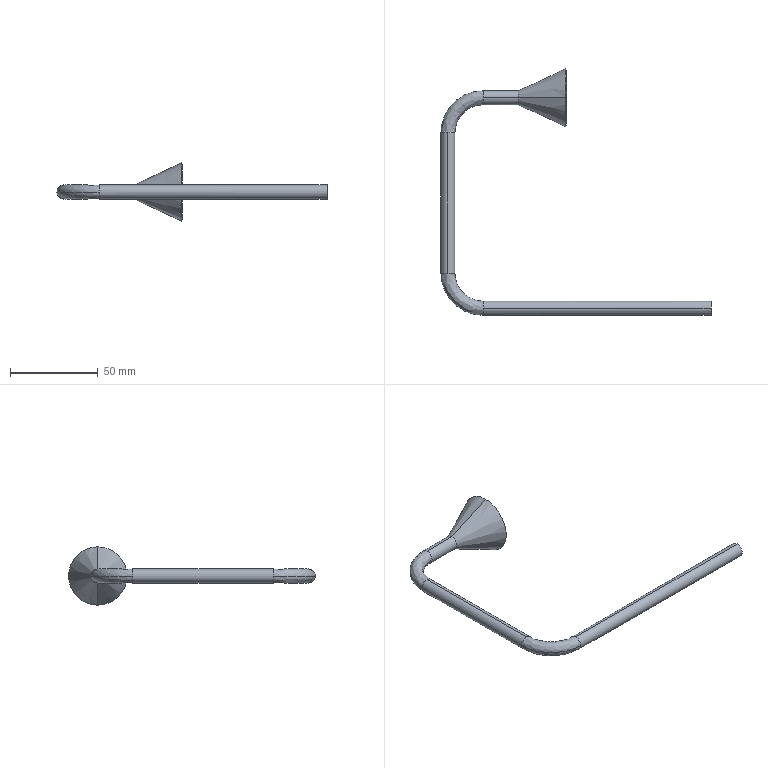Part | STEP file | 750038201 | 1 solid | 27 faces | box 154 x 140.678 x 33.357 mm | volume 8140 mm3 | cylinder 12 | spline 8 | cone 6 | plane 1 | commonest cylinder face diameters 6 x6 8 x6
STEP:
#1=CARTESIAN_POINT('',(20.,4.,0.));
#2=VERTEX_POINT('',#1);
#3=CARTESIAN_POINT('',(20.,0.,4.));
#4=VERTEX_POINT('',#3);
#5=CARTESIAN_POINT('',(20.,0.,0.));
#6=DIRECTION('',(1.,0.,0.));
#7=DIRECTION('',(0.,0.,-1.));
#8=AXIS2_PLACEMENT_3D('',#5,#6,#7);
#9=CIRCLE('',#8,4.);
#10=EDGE_CURVE('',#2,#4,#9,.T.);
#11=ORIENTED_EDGE('',*,*,#10,.T.);
#12=CARTESIAN_POINT('',(150.,0.,4.));
#13=VERTEX_POINT('',#12);
#14=CARTESIAN_POINT('',(20.,0.,4.));
#15=DIRECTION('',(1.,0.,0.));
#16=VECTOR('',#15,1000.);
#17=LINE('',#14,#16);
#18=EDGE_CURVE('',#4,#13,#17,.T.);
#19=ORIENTED_EDGE('',*,*,#18,.T.);
#20=CARTESIAN_POINT('',(150.,0.,-4.));
#21=VERTEX_POINT('',#20);
#22=CARTESIAN_POINT('',(150.,0.,0.));
#23=DIRECTION('',(-1.,0.,0.));
#24=DIRECTION('',(0.,0.,-1.));
#25=AXIS2_PLACEMENT_3D('',#22,#23,#24);
#26=CIRCLE('',#25,4.);
#27=EDGE_CURVE('',#13,#21,#26,.T.);
#28=ORIENTED_EDGE('',*,*,#27,.T.);
#29=CARTESIAN_POINT('',(20.,0.,-4.));
#30=VERTEX_POINT('',#29);
#31=CARTESIAN_POINT('',(20.,0.,-4.));
#32=DIRECTION('',(1.,0.,0.));
#33=VECTOR('',#32,1000.);
#34=LINE('',#31,#33);
#35=EDGE_CURVE('',#30,#21,#34,.T.);
#36=ORIENTED_EDGE('',*,*,#35,.F.);
#37=CARTESIAN_POINT('',(20.,0.,0.));
#38=DIRECTION('',(1.,0.,0.));
#39=DIRECTION('',(0.,0.,-1.));
#40=AXIS2_PLACEMENT_3D('',#37,#38,#39);
#41=CIRCLE('',#40,4.);
#42=EDGE_CURVE('',#30,#2,#41,.T.);
#43=ORIENTED_EDGE('',*,*,#42,.T.);
#44=EDGE_LOOP('',(#11,#19,#28,#36,#43));
#45=FACE_OUTER_BOUND('',#44,.T.);
#46=CARTESIAN_POINT('',(20.,0.,0.));
#47=DIRECTION('',(1.,0.,0.));
#48=DIRECTION('',(0.,0.,-1.));
#49=AXIS2_PLACEMENT_3D('',#46,#47,#48);
#50=CYLINDRICAL_SURFACE('',#49,4.);
#51=ADVANCED_FACE('',(#45),#50,.T.);
#52=ORIENTED_EDGE('',*,*,#10,.F.);
#53=CARTESIAN_POINT('',(4.,20.,0.));
#54=VERTEX_POINT('',#53);
#55=CARTESIAN_POINT('',(20.,20.,0.));
#56=DIRECTION('',(0.,0.,-1.));
#57=DIRECTION('',(-1.,0.,0.));
#58=AXIS2_PLACEMENT_3D('',#55,#56,#57);
#59=CIRCLE('',#58,16.);
#60=EDGE_CURVE('',#2,#54,#59,.T.);
#61=ORIENTED_EDGE('',*,*,#60,.T.);
#62=CARTESIAN_POINT('',(0.,20.,4.));
#63=VERTEX_POINT('',#62);
#64=CARTESIAN_POINT('',(0.,20.,0.));
#65=DIRECTION('',(0.,-1.,0.));
#66=DIRECTION('',(-1.,0.,0.));
#67=AXIS2_PLACEMENT_3D('',#64,#65,#66);
#68=CIRCLE('',#67,4.);
#69=EDGE_CURVE('',#54,#63,#68,.T.);
#70=ORIENTED_EDGE('',*,*,#69,.T.);
#71=CARTESIAN_POINT('',(-4.,20.,0.));
#72=VERTEX_POINT('',#71);
#73=CARTESIAN_POINT('',(0.,20.,0.));
#74=DIRECTION('',(0.,-1.,0.));
#75=DIRECTION('',(-1.,0.,0.));
#76=AXIS2_PLACEMENT_3D('',#73,#74,#75);
#77=CIRCLE('',#76,4.);
#78=EDGE_CURVE('',#63,#72,#77,.T.);
#79=ORIENTED_EDGE('',*,*,#78,.T.);
#80=CARTESIAN_POINT('',(20.,-4.,0.));
#81=VERTEX_POINT('',#80);
#82=CARTESIAN_POINT('',(20.,20.,0.));
#83=DIRECTION('',(0.,0.,-1.));
#84=DIRECTION('',(-1.,0.,0.));
#85=AXIS2_PLACEMENT_3D('',#82,#83,#84);
#86=CIRCLE('',#85,24.);
#87=EDGE_CURVE('',#81,#72,#86,.T.);
#88=ORIENTED_EDGE('',*,*,#87,.F.);
#89=CARTESIAN_POINT('',(20.,0.,0.));
#90=DIRECTION('',(1.,0.,0.));
#91=DIRECTION('',(0.,0.,-1.));
#92=AXIS2_PLACEMENT_3D('',#89,#90,#91);
#93=CIRCLE('',#92,4.);
#94=EDGE_CURVE('',#4,#81,#93,.T.);
#95=ORIENTED_EDGE('',*,*,#94,.F.);
#96=EDGE_LOOP('',(#52,#61,#70,#79,#88,#95));
#97=FACE_OUTER_BOUND('',#96,.T.);
#98=CARTESIAN_POINT('',(20.,-4.,0.));
#99=CARTESIAN_POINT('',(5.941,-4.,0.));
#100=CARTESIAN_POINT('',(-4.,5.941,0.));
#101=CARTESIAN_POINT('',(-4.,20.,0.));
#102=CARTESIAN_POINT('',(20.,-4.,8.));
#103=CARTESIAN_POINT('',(5.941,-4.,8.));
#104=CARTESIAN_POINT('',(-4.,5.941,8.));
#105=CARTESIAN_POINT('',(-4.,20.,8.));
#106=CARTESIAN_POINT('',(20.,4.,8.));
#107=CARTESIAN_POINT('',(10.627,4.,8.));
#108=CARTESIAN_POINT('',(4.,10.627,8.));
#109=CARTESIAN_POINT('',(4.,20.,8.));
#110=CARTESIAN_POINT('',(20.,4.,0.));
#111=CARTESIAN_POINT('',(10.627,4.,0.));
#112=CARTESIAN_POINT('',(4.,10.627,0.));
#113=CARTESIAN_POINT('',(4.,20.,0.));
#114=(BOUNDED_SURFACE()B_SPLINE_SURFACE(3,3,((#98,#99,#100,#101),(#102,#103,#104,#105),(#106,#107,#108,#109),(#110,#111,#112,#113)),.UNSPECIFIED.,.F.,.F.,.F.)B_SPLINE_SURFACE_WITH_KNOTS((4,4),(4,4),(0.,1.),(0.,1.),.UNSPECIFIED.)GEOMETRIC_REPRESENTATION_ITEM()RATIONAL_B_SPLINE_SURFACE(((1.,0.8047,0.8047,1.),(0.3333,0.2682,0.2682,0.3333),(0.3333,0.2682,0.2682,0.3333),(1.,0.8047,0.8047,1.)))REPRESENTATION_ITEM('')SURFACE());
#115=ADVANCED_FACE('',(#97),#114,.T.);
#116=CARTESIAN_POINT('',(20.,0.,3.));
#117=VERTEX_POINT('',#116);
#118=CARTESIAN_POINT('',(20.,-3.,0.));
#119=VERTEX_POINT('',#118);
#120=CARTESIAN_POINT('',(20.,0.,0.));
#121=DIRECTION('',(1.,0.,0.));
#122=DIRECTION('',(0.,0.,-1.));
#123=AXIS2_PLACEMENT_3D('',#120,#121,#122);
#124=CIRCLE('',#123,3.);
#125=EDGE_CURVE('',#117,#119,#124,.T.);
#126=ORIENTED_EDGE('',*,*,#125,.F.);
#127=CARTESIAN_POINT('',(150.,0.,3.));
#128=VERTEX_POINT('',#127);
#129=CARTESIAN_POINT('',(20.,0.,3.));
#130=DIRECTION('',(1.,0.,0.));
#131=VECTOR('',#130,1000.);
#132=LINE('',#129,#131);
#133=EDGE_CURVE('',#117,#128,#132,.T.);
#134=ORIENTED_EDGE('',*,*,#133,.T.);
#135=CARTESIAN_POINT('',(150.,0.,-3.));
#136=VERTEX_POINT('',#135);
#137=CARTESIAN_POINT('',(150.,0.,0.));
#138=DIRECTION('',(1.,0.,0.));
#139=DIRECTION('',(0.,0.,-1.));
#140=AXIS2_PLACEMENT_3D('',#137,#138,#139);
#141=CIRCLE('',#140,3.);
#142=EDGE_CURVE('',#128,#136,#141,.T.);
#143=ORIENTED_EDGE('',*,*,#142,.T.);
#144=CARTESIAN_POINT('',(20.,0.,-3.));
#145=VERTEX_POINT('',#144);
#146=CARTESIAN_POINT('',(20.,0.,-3.));
#147=DIRECTION('',(1.,0.,0.));
#148=VECTOR('',#147,1000.);
#149=LINE('',#146,#148);
#150=EDGE_CURVE('',#145,#136,#149,.T.);
#151=ORIENTED_EDGE('',*,*,#150,.F.);
#152=CARTESIAN_POINT('',(20.,0.,0.));
#153=DIRECTION('',(1.,0.,0.));
#154=DIRECTION('',(0.,0.,-1.));
#155=AXIS2_PLACEMENT_3D('',#152,#153,#154);
#156=CIRCLE('',#155,3.);
#157=EDGE_CURVE('',#119,#145,#156,.T.);
#158=ORIENTED_EDGE('',*,*,#157,.F.);
#159=EDGE_LOOP('',(#126,#134,#143,#151,#158));
#160=FACE_OUTER_BOUND('',#159,.T.);
#161=CARTESIAN_POINT('',(20.,0.,0.));
#162=DIRECTION('',(1.,0.,0.));
#163=DIRECTION('',(0.,0.,-1.));
#164=AXIS2_PLACEMENT_3D('',#161,#162,#163);
#165=CYLINDRICAL_SURFACE('',#164,3.);
#166=ADVANCED_FACE('',(#160),#165,.F.);
#167=CARTESIAN_POINT('',(0.,20.,-4.));
#168=VERTEX_POINT('',#167);
#169=CARTESIAN_POINT('',(0.,20.,0.));
#170=DIRECTION('',(0.,-1.,0.));
#171=DIRECTION('',(-1.,0.,0.));
#172=AXIS2_PLACEMENT_3D('',#169,#170,#171);
#173=CIRCLE('',#172,4.);
#174=EDGE_CURVE('',#168,#54,#173,.T.);
#175=ORIENTED_EDGE('',*,*,#174,.F.);
#176=CARTESIAN_POINT('',(0.,100.,-4.));
#177=VERTEX_POINT('',#176);
#178=CARTESIAN_POINT('',(0.,20.,-4.));
#179=DIRECTION('',(0.,1.,0.));
#180=VECTOR('',#179,1000.);
#181=LINE('',#178,#180);
#182=EDGE_CURVE('',#168,#177,#181,.T.);
#183=ORIENTED_EDGE('',*,*,#182,.T.);
#184=CARTESIAN_POINT('',(4.,100.,0.));
#185=VERTEX_POINT('',#184);
#186=CARTESIAN_POINT('',(0.,100.,0.));
#187=DIRECTION('',(0.,-1.,0.));
#188=DIRECTION('',(0.,0.,1.));
#189=AXIS2_PLACEMENT_3D('',#186,#187,#188);
#190=CIRCLE('',#189,4.);
#191=EDGE_CURVE('',#177,#185,#190,.T.);
#192=ORIENTED_EDGE('',*,*,#191,.T.);
#193=CARTESIAN_POINT('',(0.,100.,4.));
#194=VERTEX_POINT('',#193);
#195=CARTESIAN_POINT('',(0.,100.,0.));
#196=DIRECTION('',(0.,-1.,0.));
#197=DIRECTION('',(0.,0.,1.));
#198=AXIS2_PLACEMENT_3D('',#195,#196,#197);
#199=CIRCLE('',#198,4.);
#200=EDGE_CURVE('',#185,#194,#199,.T.);
#201=ORIENTED_EDGE('',*,*,#200,.T.);
#202=CARTESIAN_POINT('',(0.,20.,4.));
#203=DIRECTION('',(0.,1.,0.));
#204=VECTOR('',#203,1000.);
#205=LINE('',#202,#204);
#206=EDGE_CURVE('',#63,#194,#205,.T.);
#207=ORIENTED_EDGE('',*,*,#206,.F.);
#208=ORIENTED_EDGE('',*,*,#69,.F.);
#209=EDGE_LOOP('',(#175,#183,#192,#201,#207,#208));
#210=FACE_OUTER_BOUND('',#209,.T.);
#211=CARTESIAN_POINT('',(0.,20.,0.));
#212=DIRECTION('',(0.,1.,0.));
#213=DIRECTION('',(0.,0.,1.));
#214=AXIS2_PLACEMENT_3D('',#211,#212,#213);
#215=CYLINDRICAL_SURFACE('',#214,4.);
#216=ADVANCED_FACE('',(#210),#215,.T.);
#217=ORIENTED_EDGE('',*,*,#157,.T.);
#218=CARTESIAN_POINT('',(20.,3.,0.));
#219=VERTEX_POINT('',#218);
#220=CARTESIAN_POINT('',(20.,0.,0.));
#221=DIRECTION('',(1.,0.,0.));
#222=DIRECTION('',(0.,0.,-1.));
#223=AXIS2_PLACEMENT_3D('',#220,#221,#222);
#224=CIRCLE('',#223,3.);
#225=EDGE_CURVE('',#145,#219,#224,.T.);
#226=ORIENTED_EDGE('',*,*,#225,.T.);
#227=CARTESIAN_POINT('',(3.,20.,0.));
#228=VERTEX_POINT('',#227);
#229=CARTESIAN_POINT('',(20.,20.,0.));
#230=DIRECTION('',(0.,0.,-1.));
#231=DIRECTION('',(-1.,0.,0.));
#232=AXIS2_PLACEMENT_3D('',#229,#230,#231);
#233=CIRCLE('',#232,17.);
#234=EDGE_CURVE('',#219,#228,#233,.T.);
#235=ORIENTED_EDGE('',*,*,#234,.T.);
#236=CARTESIAN_POINT('',(0.,20.,-3.));
#237=VERTEX_POINT('',#236);
#238=CARTESIAN_POINT('',(0.,20.,0.));
#239=DIRECTION('',(0.,-1.,0.));
#240=DIRECTION('',(-1.,0.,0.));
#241=AXIS2_PLACEMENT_3D('',#238,#239,#240);
#242=CIRCLE('',#241,3.);
#243=EDGE_CURVE('',#237,#228,#242,.T.);
#244=ORIENTED_EDGE('',*,*,#243,.F.);
#245=CARTESIAN_POINT('',(-3.,20.,0.));
#246=VERTEX_POINT('',#245);
#247=CARTESIAN_POINT('',(0.,20.,0.));
#248=DIRECTION('',(0.,-1.,0.));
#249=DIRECTION('',(-1.,0.,0.));
#250=AXIS2_PLACEMENT_3D('',#247,#248,#249);
#251=CIRCLE('',#250,3.);
#252=EDGE_CURVE('',#246,#237,#251,.T.);
#253=ORIENTED_EDGE('',*,*,#252,.F.);
#254=CARTESIAN_POINT('',(20.,20.,0.));
#255=DIRECTION('',(0.,0.,-1.));
#256=DIRECTION('',(-1.,0.,0.));
#257=AXIS2_PLACEMENT_3D('',#254,#255,#256);
#258=CIRCLE('',#257,23.);
#259=EDGE_CURVE('',#119,#246,#258,.T.);
#260=ORIENTED_EDGE('',*,*,#259,.F.);
#261=EDGE_LOOP('',(#217,#226,#235,#244,#253,#260));
#262=FACE_OUTER_BOUND('',#261,.T.);
#263=CARTESIAN_POINT('',(20.,3.,0.));
#264=CARTESIAN_POINT('',(10.042,3.,0.));
#265=CARTESIAN_POINT('',(3.,10.042,0.));
#266=CARTESIAN_POINT('',(3.,20.,0.));
#267=CARTESIAN_POINT('',(20.,3.,-6.));
#268=CARTESIAN_POINT('',(10.042,3.,-6.));
#269=CARTESIAN_POINT('',(3.,10.042,-6.));
#270=CARTESIAN_POINT('',(3.,20.,-6.));
#271=CARTESIAN_POINT('',(20.,-3.,-6.));
#272=CARTESIAN_POINT('',(6.527,-3.,-6.));
#273=CARTESIAN_POINT('',(-3.,6.527,-6.));
#274=CARTESIAN_POINT('',(-3.,20.,-6.));
#275=CARTESIAN_POINT('',(20.,-3.,0.));
#276=CARTESIAN_POINT('',(6.527,-3.,0.));
#277=CARTESIAN_POINT('',(-3.,6.527,0.));
#278=CARTESIAN_POINT('',(-3.,20.,0.));
#279=(BOUNDED_SURFACE()B_SPLINE_SURFACE(3,3,((#263,#264,#265,#266),(#267,#268,#269,#270),(#271,#272,#273,#274),(#275,#276,#277,#278)),.UNSPECIFIED.,.F.,.F.,.F.)B_SPLINE_SURFACE_WITH_KNOTS((4,4),(4,4),(0.,1.),(0.,1.),.UNSPECIFIED.)GEOMETRIC_REPRESENTATION_ITEM()RATIONAL_B_SPLINE_SURFACE(((1.,0.8047,0.8047,1.),(0.3333,0.2682,0.2682,0.3333),(0.3333,0.2682,0.2682,0.3333),(1.,0.8047,0.8047,1.)))REPRESENTATION_ITEM('')SURFACE());
#280=ADVANCED_FACE('',(#262),#279,.F.);
#281=ORIENTED_EDGE('',*,*,#200,.F.);
#282=CARTESIAN_POINT('',(20.,116.,0.));
#283=VERTEX_POINT('',#282);
#284=CARTESIAN_POINT('',(20.,100.,0.));
#285=DIRECTION('',(0.,0.,-1.));
#286=DIRECTION('',(-1.,0.,0.));
#287=AXIS2_PLACEMENT_3D('',#284,#285,#286);
#288=CIRCLE('',#287,16.);
#289=EDGE_CURVE('',#185,#283,#288,.T.);
#290=ORIENTED_EDGE('',*,*,#289,.T.);
#291=CARTESIAN_POINT('',(20.,120.,4.));
#292=VERTEX_POINT('',#291);
#293=CARTESIAN_POINT('',(20.,120.,0.));
#294=DIRECTION('',(-1.,0.,0.));
#295=DIRECTION('',(0.,1.,0.));
#296=AXIS2_PLACEMENT_3D('',#293,#294,#295);
#297=CIRCLE('',#296,4.);
#298=EDGE_CURVE('',#283,#292,#297,.T.);
#299=ORIENTED_EDGE('',*,*,#298,.T.);
#300=CARTESIAN_POINT('',(20.,124.,0.));
#301=VERTEX_POINT('',#300);
#302=CARTESIAN_POINT('',(20.,120.,0.));
#303=DIRECTION('',(-1.,0.,0.));
#304=DIRECTION('',(0.,1.,0.));
#305=AXIS2_PLACEMENT_3D('',#302,#303,#304);
#306=CIRCLE('',#305,4.);
#307=EDGE_CURVE('',#292,#301,#306,.T.);
#308=ORIENTED_EDGE('',*,*,#307,.T.);
#309=CARTESIAN_POINT('',(-4.,100.,0.));
#310=VERTEX_POINT('',#309);
#311=CARTESIAN_POINT('',(20.,100.,0.));
#312=DIRECTION('',(0.,0.,-1.));
#313=DIRECTION('',(-1.,0.,0.));
#314=AXIS2_PLACEMENT_3D('',#311,#312,#313);
#315=CIRCLE('',#314,24.);
#316=EDGE_CURVE('',#310,#301,#315,.T.);
#317=ORIENTED_EDGE('',*,*,#316,.F.);
#318=CARTESIAN_POINT('',(0.,100.,0.));
#319=DIRECTION('',(0.,-1.,0.));
#320=DIRECTION('',(0.,0.,1.));
#321=AXIS2_PLACEMENT_3D('',#318,#319,#320);
#322=CIRCLE('',#321,4.);
#323=EDGE_CURVE('',#194,#310,#322,.T.);
#324=ORIENTED_EDGE('',*,*,#323,.F.);
#325=EDGE_LOOP('',(#281,#290,#299,#308,#317,#324));
#326=FACE_OUTER_BOUND('',#325,.T.);
#327=CARTESIAN_POINT('',(-4.,100.,0.));
#328=CARTESIAN_POINT('',(-4.,114.059,0.));
#329=CARTESIAN_POINT('',(5.941,124.,0.));
#330=CARTESIAN_POINT('',(20.,124.,0.));
#331=CARTESIAN_POINT('',(-4.,100.,8.));
#332=CARTESIAN_POINT('',(-4.,114.059,8.));
#333=CARTESIAN_POINT('',(5.941,124.,8.));
#334=CARTESIAN_POINT('',(20.,124.,8.));
#335=CARTESIAN_POINT('',(4.,100.,8.));
#336=CARTESIAN_POINT('',(4.,109.373,8.));
#337=CARTESIAN_POINT('',(10.627,116.,8.));
#338=CARTESIAN_POINT('',(20.,116.,8.));
#339=CARTESIAN_POINT('',(4.,100.,0.));
#340=CARTESIAN_POINT('',(4.,109.373,0.));
#341=CARTESIAN_POINT('',(10.627,116.,0.));
#342=CARTESIAN_POINT('',(20.,116.,0.));
#343=(BOUNDED_SURFACE()B_SPLINE_SURFACE(3,3,((#327,#328,#329,#330),(#331,#332,#333,#334),(#335,#336,#337,#338),(#339,#340,#341,#342)),.UNSPECIFIED.,.F.,.F.,.F.)B_SPLINE_SURFACE_WITH_KNOTS((4,4),(4,4),(0.,1.),(0.,1.),.UNSPECIFIED.)GEOMETRIC_REPRESENTATION_ITEM()RATIONAL_B_SPLINE_SURFACE(((1.,0.8047,0.8047,1.),(0.3333,0.2682,0.2682,0.3333),(0.3333,0.2682,0.2682,0.3333),(1.,0.8047,0.8047,1.)))REPRESENTATION_ITEM('')SURFACE());
#344=ADVANCED_FACE('',(#326),#343,.T.);
#345=CARTESIAN_POINT('',(0.,20.,3.));
#346=VERTEX_POINT('',#345);
#347=CARTESIAN_POINT('',(0.,20.,0.));
#348=DIRECTION('',(0.,-1.,0.));
#349=DIRECTION('',(-1.,0.,0.));
#350=AXIS2_PLACEMENT_3D('',#347,#348,#349);
#351=CIRCLE('',#350,3.);
#352=EDGE_CURVE('',#346,#246,#351,.T.);
#353=ORIENTED_EDGE('',*,*,#352,.T.);
#354=ORIENTED_EDGE('',*,*,#252,.T.);
#355=CARTESIAN_POINT('',(0.,100.,-3.));
#356=VERTEX_POINT('',#355);
#357=CARTESIAN_POINT('',(0.,20.,-3.));
#358=DIRECTION('',(0.,1.,0.));
#359=VECTOR('',#358,1000.);
#360=LINE('',#357,#359);
#361=EDGE_CURVE('',#237,#356,#360,.T.);
#362=ORIENTED_EDGE('',*,*,#361,.T.);
#363=CARTESIAN_POINT('',(-3.,100.,0.));
#364=VERTEX_POINT('',#363);
#365=CARTESIAN_POINT('',(0.,100.,0.));
#366=DIRECTION('',(0.,-1.,0.));
#367=DIRECTION('',(0.,0.,1.));
#368=AXIS2_PLACEMENT_3D('',#365,#366,#367);
#369=CIRCLE('',#368,3.);
#370=EDGE_CURVE('',#364,#356,#369,.T.);
#371=ORIENTED_EDGE('',*,*,#370,.F.);
#372=CARTESIAN_POINT('',(0.,100.,3.));
#373=VERTEX_POINT('',#372);
#374=CARTESIAN_POINT('',(0.,100.,0.));
#375=DIRECTION('',(0.,-1.,0.));
#376=DIRECTION('',(0.,0.,1.));
#377=AXIS2_PLACEMENT_3D('',#374,#375,#376);
#378=CIRCLE('',#377,3.);
#379=EDGE_CURVE('',#373,#364,#378,.T.);
#380=ORIENTED_EDGE('',*,*,#379,.F.);
#381=CARTESIAN_POINT('',(0.,20.,3.));
#382=DIRECTION('',(0.,1.,0.));
#383=VECTOR('',#382,1000.);
#384=LINE('',#381,#383);
#385=EDGE_CURVE('',#346,#373,#384,.T.);
#386=ORIENTED_EDGE('',*,*,#385,.F.);
#387=EDGE_LOOP('',(#353,#354,#362,#371,#380,#386));
#388=FACE_OUTER_BOUND('',#387,.T.);
#389=CARTESIAN_POINT('',(0.,20.,0.));
#390=DIRECTION('',(0.,1.,0.));
#391=DIRECTION('',(0.,0.,1.));
#392=AXIS2_PLACEMENT_3D('',#389,#390,#391);
#393=CYLINDRICAL_SURFACE('',#392,3.);
#394=ADVANCED_FACE('',(#388),#393,.F.);
#395=ORIENTED_EDGE('',*,*,#307,.F.);
#396=CARTESIAN_POINT('',(40.,120.,4.));
#397=VERTEX_POINT('',#396);
#398=CARTESIAN_POINT('',(20.,120.,4.));
#399=DIRECTION('',(1.,0.,0.));
#400=VECTOR('',#399,1000.);
#401=LINE('',#398,#400);
#402=EDGE_CURVE('',#292,#397,#401,.T.);
#403=ORIENTED_EDGE('',*,*,#402,.T.);
#404=CARTESIAN_POINT('',(40.,120.,-4.));
#405=VERTEX_POINT('',#404);
#406=CARTESIAN_POINT('',(40.,120.,0.));
#407=DIRECTION('',(-1.,0.,0.));
#408=DIRECTION('',(0.,0.,-1.));
#409=AXIS2_PLACEMENT_3D('',#406,#407,#408);
#410=CIRCLE('',#409,4.);
#411=EDGE_CURVE('',#397,#405,#410,.T.);
#412=ORIENTED_EDGE('',*,*,#411,.T.);
#413=CARTESIAN_POINT('',(20.,120.,-4.));
#414=VERTEX_POINT('',#413);
#415=CARTESIAN_POINT('',(20.,120.,-4.));
#416=DIRECTION('',(1.,0.,0.));
#417=VECTOR('',#416,1000.);
#418=LINE('',#415,#417);
#419=EDGE_CURVE('',#414,#405,#418,.T.);
#420=ORIENTED_EDGE('',*,*,#419,.F.);
#421=CARTESIAN_POINT('',(20.,120.,0.));
#422=DIRECTION('',(-1.,0.,0.));
#423=DIRECTION('',(0.,1.,0.));
#424=AXIS2_PLACEMENT_3D('',#421,#422,#423);
#425=CIRCLE('',#424,4.);
#426=EDGE_CURVE('',#301,#414,#425,.T.);
#427=ORIENTED_EDGE('',*,*,#426,.F.);
#428=EDGE_LOOP('',(#395,#403,#412,#420,#427));
#429=FACE_OUTER_BOUND('',#428,.T.);
#430=CARTESIAN_POINT('',(20.,120.,0.));
#431=DIRECTION('',(1.,0.,0.));
#432=DIRECTION('',(0.,0.,-1.));
#433=AXIS2_PLACEMENT_3D('',#430,#431,#432);
#434=CYLINDRICAL_SURFACE('',#433,4.);
#435=ADVANCED_FACE('',(#429),#434,.T.);
#436=ORIENTED_EDGE('',*,*,#370,.T.);
#437=CARTESIAN_POINT('',(3.,100.,0.));
#438=VERTEX_POINT('',#437);
#439=CARTESIAN_POINT('',(0.,100.,0.));
#440=DIRECTION('',(0.,-1.,0.));
#441=DIRECTION('',(0.,0.,1.));
#442=AXIS2_PLACEMENT_3D('',#439,#440,#441);
#443=CIRCLE('',#442,3.);
#444=EDGE_CURVE('',#356,#438,#443,.T.);
#445=ORIENTED_EDGE('',*,*,#444,.T.);
#446=CARTESIAN_POINT('',(20.,117.,0.));
#447=VERTEX_POINT('',#446);
#448=CARTESIAN_POINT('',(20.,100.,0.));
#449=DIRECTION('',(0.,0.,-1.));
#450=DIRECTION('',(-1.,0.,0.));
#451=AXIS2_PLACEMENT_3D('',#448,#449,#450);
#452=CIRCLE('',#451,17.);
#453=EDGE_CURVE('',#438,#447,#452,.T.);
#454=ORIENTED_EDGE('',*,*,#453,.T.);
#455=CARTESIAN_POINT('',(20.,120.,-3.));
#456=VERTEX_POINT('',#455);
#457=CARTESIAN_POINT('',(20.,120.,0.));
#458=DIRECTION('',(-1.,0.,0.));
#459=DIRECTION('',(0.,1.,0.));
#460=AXIS2_PLACEMENT_3D('',#457,#458,#459);
#461=CIRCLE('',#460,3.);
#462=EDGE_CURVE('',#456,#447,#461,.T.);
#463=ORIENTED_EDGE('',*,*,#462,.F.);
#464=CARTESIAN_POINT('',(20.,123.,0.));
#465=VERTEX_POINT('',#464);
#466=CARTESIAN_POINT('',(20.,120.,0.));
#467=DIRECTION('',(-1.,0.,0.));
#468=DIRECTION('',(0.,1.,0.));
#469=AXIS2_PLACEMENT_3D('',#466,#467,#468);
#470=CIRCLE('',#469,3.);
#471=EDGE_CURVE('',#465,#456,#470,.T.);
#472=ORIENTED_EDGE('',*,*,#471,.F.);
#473=CARTESIAN_POINT('',(20.,100.,0.));
#474=DIRECTION('',(0.,0.,-1.));
#475=DIRECTION('',(-1.,0.,0.));
#476=AXIS2_PLACEMENT_3D('',#473,#474,#475);
#477=CIRCLE('',#476,23.);
#478=EDGE_CURVE('',#364,#465,#477,.T.);
#479=ORIENTED_EDGE('',*,*,#478,.F.);
#480=EDGE_LOOP('',(#436,#445,#454,#463,#472,#479));
#481=FACE_OUTER_BOUND('',#480,.T.);
#482=CARTESIAN_POINT('',(3.,100.,0.));
#483=CARTESIAN_POINT('',(3.,109.958,0.));
#484=CARTESIAN_POINT('',(10.042,117.,0.));
#485=CARTESIAN_POINT('',(20.,117.,0.));
#486=CARTESIAN_POINT('',(3.,100.,-6.));
#487=CARTESIAN_POINT('',(3.,109.958,-6.));
#488=CARTESIAN_POINT('',(10.042,117.,-6.));
#489=CARTESIAN_POINT('',(20.,117.,-6.));
#490=CARTESIAN_POINT('',(-3.,100.,-6.));
#491=CARTESIAN_POINT('',(-3.,113.473,-6.));
#492=CARTESIAN_POINT('',(6.527,123.,-6.));
#493=CARTESIAN_POINT('',(20.,123.,-6.));
#494=CARTESIAN_POINT('',(-3.,100.,0.));
#495=CARTESIAN_POINT('',(-3.,113.473,0.));
#496=CARTESIAN_POINT('',(6.527,123.,0.));
#497=CARTESIAN_POINT('',(20.,123.,0.));
#498=(BOUNDED_SURFACE()B_SPLINE_SURFACE(3,3,((#482,#483,#484,#485),(#486,#487,#488,#489),(#490,#491,#492,#493),(#494,#495,#496,#497)),.UNSPECIFIED.,.F.,.F.,.F.)B_SPLINE_SURFACE_WITH_KNOTS((4,4),(4,4),(0.,1.),(0.,1.),.UNSPECIFIED.)GEOMETRIC_REPRESENTATION_ITEM()RATIONAL_B_SPLINE_SURFACE(((1.,0.8047,0.8047,1.),(0.3333,0.2682,0.2682,0.3333),(0.3333,0.2682,0.2682,0.3333),(1.,0.8047,0.8047,1.)))REPRESENTATION_ITEM('')SURFACE());
#499=ADVANCED_FACE('',(#481),#498,.F.);
#500=ORIENTED_EDGE('',*,*,#462,.T.);
#501=CARTESIAN_POINT('',(20.,120.,3.));
#502=VERTEX_POINT('',#501);
#503=CARTESIAN_POINT('',(20.,120.,0.));
#504=DIRECTION('',(-1.,0.,0.));
#505=DIRECTION('',(0.,1.,0.));
#506=AXIS2_PLACEMENT_3D('',#503,#504,#505);
#507=CIRCLE('',#506,3.);
#508=EDGE_CURVE('',#447,#502,#507,.T.);
#509=ORIENTED_EDGE('',*,*,#508,.T.);
#510=CARTESIAN_POINT('',(40.,120.,3.));
#511=VERTEX_POINT('',#510);
#512=CARTESIAN_POINT('',(20.,120.,3.));
#513=DIRECTION('',(1.,0.,0.));
#514=VECTOR('',#513,1000.);
#515=LINE('',#512,#514);
#516=EDGE_CURVE('',#502,#511,#515,.T.);
#517=ORIENTED_EDGE('',*,*,#516,.T.);
#518=CARTESIAN_POINT('',(40.,120.,-3.));
#519=VERTEX_POINT('',#518);
#520=CARTESIAN_POINT('',(40.,120.,0.));
#521=DIRECTION('',(-1.,0.,0.));
#522=DIRECTION('',(0.,0.,-1.));
#523=AXIS2_PLACEMENT_3D('',#520,#521,#522);
#524=CIRCLE('',#523,3.);
#525=EDGE_CURVE('',#519,#511,#524,.T.);
#526=ORIENTED_EDGE('',*,*,#525,.F.);
#527=CARTESIAN_POINT('',(20.,120.,-3.));
#528=DIRECTION('',(1.,0.,0.));
#529=VECTOR('',#528,1000.);
#530=LINE('',#527,#529);
#531=EDGE_CURVE('',#456,#519,#530,.T.);
#532=ORIENTED_EDGE('',*,*,#531,.F.);
#533=EDGE_LOOP('',(#500,#509,#517,#526,#532));
#534=FACE_OUTER_BOUND('',#533,.T.);
#535=CARTESIAN_POINT('',(20.,120.,0.));
#536=DIRECTION('',(1.,0.,0.));
#537=DIRECTION('',(0.,0.,-1.));
#538=AXIS2_PLACEMENT_3D('',#535,#536,#537);
#539=CYLINDRICAL_SURFACE('',#538,3.);
#540=ADVANCED_FACE('',(#534),#539,.F.);
#541=ORIENTED_EDGE('',*,*,#525,.T.);
#542=CARTESIAN_POINT('',(67.572,120.,15.857));
#543=VERTEX_POINT('',#542);
#544=CARTESIAN_POINT('',(67.572,120.,15.857));
#545=DIRECTION('',(0.9063,0.,0.4226));
#546=VECTOR('',#545,1000.);
#547=LINE('',#544,#546);
#548=EDGE_CURVE('',#511,#543,#547,.T.);
#549=ORIENTED_EDGE('',*,*,#548,.T.);
#550=CARTESIAN_POINT('',(67.572,120.,-15.857));
#551=VERTEX_POINT('',#550);
#552=CARTESIAN_POINT('',(67.572,120.,0.));
#553=DIRECTION('',(-1.,0.,0.));
#554=DIRECTION('',(0.,0.,-1.));
#555=AXIS2_PLACEMENT_3D('',#552,#553,#554);
#556=CIRCLE('',#555,15.857);
#557=EDGE_CURVE('',#551,#543,#556,.T.);
#558=ORIENTED_EDGE('',*,*,#557,.F.);
#559=CARTESIAN_POINT('',(67.572,120.,-15.857));
#560=DIRECTION('',(0.9063,0.,-0.4226));
#561=VECTOR('',#560,1000.);
#562=LINE('',#559,#561);
#563=EDGE_CURVE('',#519,#551,#562,.T.);
#564=ORIENTED_EDGE('',*,*,#563,.F.);
#565=EDGE_LOOP('',(#541,#549,#558,#564));
#566=FACE_OUTER_BOUND('',#565,.T.);
#567=CARTESIAN_POINT('',(67.572,120.,0.));
#568=DIRECTION('',(1.,0.,0.));
#569=DIRECTION('',(0.,0.,-1.));
#570=AXIS2_PLACEMENT_3D('',#567,#568,#569);
#571=CONICAL_SURFACE('',#570,15.857,0.4363);
#572=ADVANCED_FACE('',(#566),#571,.F.);
#573=CARTESIAN_POINT('',(67.572,120.,0.));
#574=DIRECTION('',(-1.,0.,0.));
#575=DIRECTION('',(0.,0.,-1.));
#576=AXIS2_PLACEMENT_3D('',#573,#574,#575);
#577=CIRCLE('',#576,15.857);
#578=EDGE_CURVE('',#543,#551,#577,.T.);
#579=ORIENTED_EDGE('',*,*,#578,.T.);
#580=CARTESIAN_POINT('',(67.189,120.,-16.678));
#581=VERTEX_POINT('',#580);
#582=CARTESIAN_POINT('',(67.189,120.,-16.678));
#583=DIRECTION('',(-0.4226,0.,-0.9063));
#584=VECTOR('',#583,1000.);
#585=LINE('',#582,#584);
#586=EDGE_CURVE('',#551,#581,#585,.T.);
#587=ORIENTED_EDGE('',*,*,#586,.T.);
#588=CARTESIAN_POINT('',(67.189,120.,16.678));
#589=VERTEX_POINT('',#588);
#590=CARTESIAN_POINT('',(67.189,120.,0.));
#591=DIRECTION('',(1.,0.,0.));
#592=DIRECTION('',(0.,0.,1.));
#593=AXIS2_PLACEMENT_3D('',#590,#591,#592);
#594=CIRCLE('',#593,16.678);
#595=EDGE_CURVE('',#581,#589,#594,.T.);
#596=ORIENTED_EDGE('',*,*,#595,.T.);
#597=CARTESIAN_POINT('',(67.189,120.,16.678));
#598=DIRECTION('',(-0.4226,0.,0.9063));
#599=VECTOR('',#598,1000.);
#600=LINE('',#597,#599);
#601=EDGE_CURVE('',#543,#589,#600,.T.);
#602=ORIENTED_EDGE('',*,*,#601,.F.);
#603=EDGE_LOOP('',(#579,#587,#596,#602));
#604=FACE_OUTER_BOUND('',#603,.T.);
#605=CARTESIAN_POINT('',(67.189,120.,0.));
#606=DIRECTION('',(-1.,0.,0.));
#607=DIRECTION('',(0.,0.,1.));
#608=AXIS2_PLACEMENT_3D('',#605,#606,#607);
#609=CONICAL_SURFACE('',#608,16.678,1.134);
#610=ADVANCED_FACE('',(#604),#609,.T.);
#611=ORIENTED_EDGE('',*,*,#411,.F.);
#612=CARTESIAN_POINT('',(67.189,120.,16.678));
#613=DIRECTION('',(0.9063,0.,0.4226));
#614=VECTOR('',#613,1000.);
#615=LINE('',#612,#614);
#616=EDGE_CURVE('',#397,#589,#615,.T.);
#617=ORIENTED_EDGE('',*,*,#616,.T.);
#618=ORIENTED_EDGE('',*,*,#595,.F.);
#619=CARTESIAN_POINT('',(67.189,120.,-16.678));
#620=DIRECTION('',(0.9063,0.,-0.4226));
#621=VECTOR('',#620,1000.);
#622=LINE('',#619,#621);
#623=EDGE_CURVE('',#405,#581,#622,.T.);
#624=ORIENTED_EDGE('',*,*,#623,.F.);
#625=EDGE_LOOP('',(#611,#617,#618,#624));
#626=FACE_OUTER_BOUND('',#625,.T.);
#627=CARTESIAN_POINT('',(67.189,120.,0.));
#628=DIRECTION('',(1.,0.,0.));
#629=DIRECTION('',(0.,0.,-1.));
#630=AXIS2_PLACEMENT_3D('',#627,#628,#629);
#631=CONICAL_SURFACE('',#630,16.678,0.4363);
#632=ADVANCED_FACE('',(#626),#631,.T.);
#633=ORIENTED_EDGE('',*,*,#18,.F.);
#634=ORIENTED_EDGE('',*,*,#94,.T.);
#635=CARTESIAN_POINT('',(20.,0.,0.));
#636=DIRECTION('',(1.,0.,0.));
#637=DIRECTION('',(0.,0.,-1.));
#638=AXIS2_PLACEMENT_3D('',#635,#636,#637);
#639=CIRCLE('',#638,4.);
#640=EDGE_CURVE('',#81,#30,#639,.T.);
#641=ORIENTED_EDGE('',*,*,#640,.T.);
#642=ORIENTED_EDGE('',*,*,#35,.T.);
#643=CARTESIAN_POINT('',(150.,0.,0.));
#644=DIRECTION('',(-1.,0.,0.));
#645=DIRECTION('',(0.,0.,-1.));
#646=AXIS2_PLACEMENT_3D('',#643,#644,#645);
#647=CIRCLE('',#646,4.);
#648=EDGE_CURVE('',#21,#13,#647,.T.);
#649=ORIENTED_EDGE('',*,*,#648,.T.);
#650=EDGE_LOOP('',(#633,#634,#641,#642,#649));
#651=FACE_OUTER_BOUND('',#650,.T.);
#652=CARTESIAN_POINT('',(20.,0.,0.));
#653=DIRECTION('',(1.,0.,0.));
#654=DIRECTION('',(0.,0.,-1.));
#655=AXIS2_PLACEMENT_3D('',#652,#653,#654);
#656=CYLINDRICAL_SURFACE('',#655,4.);
#657=ADVANCED_FACE('',(#651),#656,.T.);
#658=ORIENTED_EDGE('',*,*,#648,.F.);
#659=ORIENTED_EDGE('',*,*,#27,.F.);
#660=EDGE_LOOP('',(#658,#659));
#661=FACE_OUTER_BOUND('',#660,.T.);
#662=CARTESIAN_POINT('',(150.,0.,0.));
#663=DIRECTION('',(1.,0.,0.));
#664=DIRECTION('',(0.,0.,-1.));
#665=AXIS2_PLACEMENT_3D('',#662,#663,#664);
#666=CIRCLE('',#665,3.);
#667=EDGE_CURVE('',#136,#128,#666,.T.);
#668=ORIENTED_EDGE('',*,*,#667,.F.);
#669=ORIENTED_EDGE('',*,*,#142,.F.);
#670=EDGE_LOOP('',(#668,#669));
#671=FACE_BOUND('',#670,.T.);
#672=CARTESIAN_POINT('',(150.,0.,0.));
#673=DIRECTION('',(-1.,0.,0.));
#674=DIRECTION('',(0.,0.,1.));
#675=AXIS2_PLACEMENT_3D('',#672,#673,#674);
#676=PLANE('',#675);
#677=ADVANCED_FACE('',(#661,#671),#676,.F.);
#678=ORIENTED_EDGE('',*,*,#60,.F.);
#679=ORIENTED_EDGE('',*,*,#42,.F.);
#680=ORIENTED_EDGE('',*,*,#640,.F.);
#681=ORIENTED_EDGE('',*,*,#87,.T.);
#682=CARTESIAN_POINT('',(0.,20.,0.));
#683=DIRECTION('',(0.,-1.,0.));
#684=DIRECTION('',(-1.,0.,0.));
#685=AXIS2_PLACEMENT_3D('',#682,#683,#684);
#686=CIRCLE('',#685,4.);
#687=EDGE_CURVE('',#72,#168,#686,.T.);
#688=ORIENTED_EDGE('',*,*,#687,.T.);
#689=ORIENTED_EDGE('',*,*,#174,.T.);
#690=EDGE_LOOP('',(#678,#679,#680,#681,#688,#689));
#691=FACE_OUTER_BOUND('',#690,.T.);
#692=CARTESIAN_POINT('',(20.,4.,0.));
#693=CARTESIAN_POINT('',(10.627,4.,0.));
#694=CARTESIAN_POINT('',(4.,10.627,0.));
#695=CARTESIAN_POINT('',(4.,20.,0.));
#696=CARTESIAN_POINT('',(20.,4.,-8.));
#697=CARTESIAN_POINT('',(10.627,4.,-8.));
#698=CARTESIAN_POINT('',(4.,10.627,-8.));
#699=CARTESIAN_POINT('',(4.,20.,-8.));
#700=CARTESIAN_POINT('',(20.,-4.,-8.));
#701=CARTESIAN_POINT('',(5.941,-4.,-8.));
#702=CARTESIAN_POINT('',(-4.,5.941,-8.));
#703=CARTESIAN_POINT('',(-4.,20.,-8.));
#704=CARTESIAN_POINT('',(20.,-4.,0.));
#705=CARTESIAN_POINT('',(5.941,-4.,0.));
#706=CARTESIAN_POINT('',(-4.,5.941,0.));
#707=CARTESIAN_POINT('',(-4.,20.,0.));
#708=(BOUNDED_SURFACE()B_SPLINE_SURFACE(3,3,((#692,#693,#694,#695),(#696,#697,#698,#699),(#700,#701,#702,#703),(#704,#705,#706,#707)),.UNSPECIFIED.,.F.,.F.,.F.)B_SPLINE_SURFACE_WITH_KNOTS((4,4),(4,4),(0.,1.),(0.,1.),.UNSPECIFIED.)GEOMETRIC_REPRESENTATION_ITEM()RATIONAL_B_SPLINE_SURFACE(((1.,0.8047,0.8047,1.),(0.3333,0.2682,0.2682,0.3333),(0.3333,0.2682,0.2682,0.3333),(1.,0.8047,0.8047,1.)))REPRESENTATION_ITEM('')SURFACE());
#709=ADVANCED_FACE('',(#691),#708,.T.);
#710=ORIENTED_EDGE('',*,*,#133,.F.);
#711=CARTESIAN_POINT('',(20.,0.,0.));
#712=DIRECTION('',(1.,0.,0.));
#713=DIRECTION('',(0.,0.,-1.));
#714=AXIS2_PLACEMENT_3D('',#711,#712,#713);
#715=CIRCLE('',#714,3.);
#716=EDGE_CURVE('',#219,#117,#715,.T.);
#717=ORIENTED_EDGE('',*,*,#716,.F.);
#718=ORIENTED_EDGE('',*,*,#225,.F.);
#719=ORIENTED_EDGE('',*,*,#150,.T.);
#720=ORIENTED_EDGE('',*,*,#667,.T.);
#721=EDGE_LOOP('',(#710,#717,#718,#719,#720));
#722=FACE_OUTER_BOUND('',#721,.T.);
#723=CARTESIAN_POINT('',(20.,0.,0.));
#724=DIRECTION('',(1.,0.,0.));
#725=DIRECTION('',(0.,0.,-1.));
#726=AXIS2_PLACEMENT_3D('',#723,#724,#725);
#727=CYLINDRICAL_SURFACE('',#726,3.);
#728=ADVANCED_FACE('',(#722),#727,.F.);
#729=ORIENTED_EDGE('',*,*,#182,.F.);
#730=ORIENTED_EDGE('',*,*,#687,.F.);
#731=ORIENTED_EDGE('',*,*,#78,.F.);
#732=ORIENTED_EDGE('',*,*,#206,.T.);
#733=ORIENTED_EDGE('',*,*,#323,.T.);
#734=CARTESIAN_POINT('',(0.,100.,0.));
#735=DIRECTION('',(0.,-1.,0.));
#736=DIRECTION('',(0.,0.,1.));
#737=AXIS2_PLACEMENT_3D('',#734,#735,#736);
#738=CIRCLE('',#737,4.);
#739=EDGE_CURVE('',#310,#177,#738,.T.);
#740=ORIENTED_EDGE('',*,*,#739,.T.);
#741=EDGE_LOOP('',(#729,#730,#731,#732,#733,#740));
#742=FACE_OUTER_BOUND('',#741,.T.);
#743=CARTESIAN_POINT('',(0.,20.,0.));
#744=DIRECTION('',(0.,1.,0.));
#745=DIRECTION('',(0.,0.,1.));
#746=AXIS2_PLACEMENT_3D('',#743,#744,#745);
#747=CYLINDRICAL_SURFACE('',#746,4.);
#748=ADVANCED_FACE('',(#742),#747,.T.);
#749=ORIENTED_EDGE('',*,*,#234,.F.);
#750=ORIENTED_EDGE('',*,*,#716,.T.);
#751=ORIENTED_EDGE('',*,*,#125,.T.);
#752=ORIENTED_EDGE('',*,*,#259,.T.);
#753=ORIENTED_EDGE('',*,*,#352,.F.);
#754=CARTESIAN_POINT('',(0.,20.,0.));
#755=DIRECTION('',(0.,-1.,0.));
#756=DIRECTION('',(-1.,0.,0.));
#757=AXIS2_PLACEMENT_3D('',#754,#755,#756);
#758=CIRCLE('',#757,3.);
#759=EDGE_CURVE('',#228,#346,#758,.T.);
#760=ORIENTED_EDGE('',*,*,#759,.F.);
#761=EDGE_LOOP('',(#749,#750,#751,#752,#753,#760));
#762=FACE_OUTER_BOUND('',#761,.T.);
#763=CARTESIAN_POINT('',(20.,-3.,0.));
#764=CARTESIAN_POINT('',(6.527,-3.,0.));
#765=CARTESIAN_POINT('',(-3.,6.527,0.));
#766=CARTESIAN_POINT('',(-3.,20.,0.));
#767=CARTESIAN_POINT('',(20.,-3.,6.));
#768=CARTESIAN_POINT('',(6.527,-3.,6.));
#769=CARTESIAN_POINT('',(-3.,6.527,6.));
#770=CARTESIAN_POINT('',(-3.,20.,6.));
#771=CARTESIAN_POINT('',(20.,3.,6.));
#772=CARTESIAN_POINT('',(10.042,3.,6.));
#773=CARTESIAN_POINT('',(3.,10.042,6.));
#774=CARTESIAN_POINT('',(3.,20.,6.));
#775=CARTESIAN_POINT('',(20.,3.,0.));
#776=CARTESIAN_POINT('',(10.042,3.,0.));
#777=CARTESIAN_POINT('',(3.,10.042,0.));
#778=CARTESIAN_POINT('',(3.,20.,0.));
#779=(BOUNDED_SURFACE()B_SPLINE_SURFACE(3,3,((#763,#764,#765,#766),(#767,#768,#769,#770),(#771,#772,#773,#774),(#775,#776,#777,#778)),.UNSPECIFIED.,.F.,.F.,.F.)B_SPLINE_SURFACE_WITH_KNOTS((4,4),(4,4),(0.,1.),(0.,1.),.UNSPECIFIED.)GEOMETRIC_REPRESENTATION_ITEM()RATIONAL_B_SPLINE_SURFACE(((1.,0.8047,0.8047,1.),(0.3333,0.2682,0.2682,0.3333),(0.3333,0.2682,0.2682,0.3333),(1.,0.8047,0.8047,1.)))REPRESENTATION_ITEM('')SURFACE());
#780=ADVANCED_FACE('',(#762),#779,.F.);
#781=ORIENTED_EDGE('',*,*,#289,.F.);
#782=ORIENTED_EDGE('',*,*,#191,.F.);
#783=ORIENTED_EDGE('',*,*,#739,.F.);
#784=ORIENTED_EDGE('',*,*,#316,.T.);
#785=ORIENTED_EDGE('',*,*,#426,.T.);
#786=CARTESIAN_POINT('',(20.,120.,0.));
#787=DIRECTION('',(-1.,0.,0.));
#788=DIRECTION('',(0.,1.,0.));
#789=AXIS2_PLACEMENT_3D('',#786,#787,#788);
#790=CIRCLE('',#789,4.);
#791=EDGE_CURVE('',#414,#283,#790,.T.);
#792=ORIENTED_EDGE('',*,*,#791,.T.);
#793=EDGE_LOOP('',(#781,#782,#783,#784,#785,#792));
#794=FACE_OUTER_BOUND('',#793,.T.);
#795=CARTESIAN_POINT('',(4.,100.,0.));
#796=CARTESIAN_POINT('',(4.,109.373,0.));
#797=CARTESIAN_POINT('',(10.627,116.,0.));
#798=CARTESIAN_POINT('',(20.,116.,0.));
#799=CARTESIAN_POINT('',(4.,100.,-8.));
#800=CARTESIAN_POINT('',(4.,109.373,-8.));
#801=CARTESIAN_POINT('',(10.627,116.,-8.));
#802=CARTESIAN_POINT('',(20.,116.,-8.));
#803=CARTESIAN_POINT('',(-4.,100.,-8.));
#804=CARTESIAN_POINT('',(-4.,114.059,-8.));
#805=CARTESIAN_POINT('',(5.941,124.,-8.));
#806=CARTESIAN_POINT('',(20.,124.,-8.));
#807=CARTESIAN_POINT('',(-4.,100.,0.));
#808=CARTESIAN_POINT('',(-4.,114.059,0.));
#809=CARTESIAN_POINT('',(5.941,124.,0.));
#810=CARTESIAN_POINT('',(20.,124.,0.));
#811=(BOUNDED_SURFACE()B_SPLINE_SURFACE(3,3,((#795,#796,#797,#798),(#799,#800,#801,#802),(#803,#804,#805,#806),(#807,#808,#809,#810)),.UNSPECIFIED.,.F.,.F.,.F.)B_SPLINE_SURFACE_WITH_KNOTS((4,4),(4,4),(0.,1.),(0.,1.),.UNSPECIFIED.)GEOMETRIC_REPRESENTATION_ITEM()RATIONAL_B_SPLINE_SURFACE(((1.,0.8047,0.8047,1.),(0.3333,0.2682,0.2682,0.3333),(0.3333,0.2682,0.2682,0.3333),(1.,0.8047,0.8047,1.)))REPRESENTATION_ITEM('')SURFACE());
#812=ADVANCED_FACE('',(#794),#811,.T.);
#813=ORIENTED_EDGE('',*,*,#361,.F.);
#814=ORIENTED_EDGE('',*,*,#243,.T.);
#815=ORIENTED_EDGE('',*,*,#759,.T.);
#816=ORIENTED_EDGE('',*,*,#385,.T.);
#817=CARTESIAN_POINT('',(0.,100.,0.));
#818=DIRECTION('',(0.,-1.,0.));
#819=DIRECTION('',(0.,0.,1.));
#820=AXIS2_PLACEMENT_3D('',#817,#818,#819);
#821=CIRCLE('',#820,3.);
#822=EDGE_CURVE('',#438,#373,#821,.T.);
#823=ORIENTED_EDGE('',*,*,#822,.F.);
#824=ORIENTED_EDGE('',*,*,#444,.F.);
#825=EDGE_LOOP('',(#813,#814,#815,#816,#823,#824));
#826=FACE_OUTER_BOUND('',#825,.T.);
#827=CARTESIAN_POINT('',(0.,20.,0.));
#828=DIRECTION('',(0.,1.,0.));
#829=DIRECTION('',(0.,0.,1.));
#830=AXIS2_PLACEMENT_3D('',#827,#828,#829);
#831=CYLINDRICAL_SURFACE('',#830,3.);
#832=ADVANCED_FACE('',(#826),#831,.F.);
#833=ORIENTED_EDGE('',*,*,#402,.F.);
#834=ORIENTED_EDGE('',*,*,#298,.F.);
#835=ORIENTED_EDGE('',*,*,#791,.F.);
#836=ORIENTED_EDGE('',*,*,#419,.T.);
#837=CARTESIAN_POINT('',(40.,120.,0.));
#838=DIRECTION('',(-1.,0.,0.));
#839=DIRECTION('',(0.,0.,-1.));
#840=AXIS2_PLACEMENT_3D('',#837,#838,#839);
#841=CIRCLE('',#840,4.);
#842=EDGE_CURVE('',#405,#397,#841,.T.);
#843=ORIENTED_EDGE('',*,*,#842,.T.);
#844=EDGE_LOOP('',(#833,#834,#835,#836,#843));
#845=FACE_OUTER_BOUND('',#844,.T.);
#846=CARTESIAN_POINT('',(20.,120.,0.));
#847=DIRECTION('',(1.,0.,0.));
#848=DIRECTION('',(0.,0.,-1.));
#849=AXIS2_PLACEMENT_3D('',#846,#847,#848);
#850=CYLINDRICAL_SURFACE('',#849,4.);
#851=ADVANCED_FACE('',(#845),#850,.T.);
#852=ORIENTED_EDGE('',*,*,#453,.F.);
#853=ORIENTED_EDGE('',*,*,#822,.T.);
#854=ORIENTED_EDGE('',*,*,#379,.T.);
#855=ORIENTED_EDGE('',*,*,#478,.T.);
#856=CARTESIAN_POINT('',(20.,120.,0.));
#857=DIRECTION('',(-1.,0.,0.));
#858=DIRECTION('',(0.,1.,0.));
#859=AXIS2_PLACEMENT_3D('',#856,#857,#858);
#860=CIRCLE('',#859,3.);
#861=EDGE_CURVE('',#502,#465,#860,.T.);
#862=ORIENTED_EDGE('',*,*,#861,.F.);
#863=ORIENTED_EDGE('',*,*,#508,.F.);
#864=EDGE_LOOP('',(#852,#853,#854,#855,#862,#863));
#865=FACE_OUTER_BOUND('',#864,.T.);
#866=CARTESIAN_POINT('',(-3.,100.,0.));
#867=CARTESIAN_POINT('',(-3.,113.473,0.));
#868=CARTESIAN_POINT('',(6.527,123.,0.));
#869=CARTESIAN_POINT('',(20.,123.,0.));
#870=CARTESIAN_POINT('',(-3.,100.,6.));
#871=CARTESIAN_POINT('',(-3.,113.473,6.));
#872=CARTESIAN_POINT('',(6.527,123.,6.));
#873=CARTESIAN_POINT('',(20.,123.,6.));
#874=CARTESIAN_POINT('',(3.,100.,6.));
#875=CARTESIAN_POINT('',(3.,109.958,6.));
#876=CARTESIAN_POINT('',(10.042,117.,6.));
#877=CARTESIAN_POINT('',(20.,117.,6.));
#878=CARTESIAN_POINT('',(3.,100.,0.));
#879=CARTESIAN_POINT('',(3.,109.958,0.));
#880=CARTESIAN_POINT('',(10.042,117.,0.));
#881=CARTESIAN_POINT('',(20.,117.,0.));
#882=(BOUNDED_SURFACE()B_SPLINE_SURFACE(3,3,((#866,#867,#868,#869),(#870,#871,#872,#873),(#874,#875,#876,#877),(#878,#879,#880,#881)),.UNSPECIFIED.,.F.,.F.,.F.)B_SPLINE_SURFACE_WITH_KNOTS((4,4),(4,4),(0.,1.),(0.,1.),.UNSPECIFIED.)GEOMETRIC_REPRESENTATION_ITEM()RATIONAL_B_SPLINE_SURFACE(((1.,0.8047,0.8047,1.),(0.3333,0.2682,0.2682,0.3333),(0.3333,0.2682,0.2682,0.3333),(1.,0.8047,0.8047,1.)))REPRESENTATION_ITEM('')SURFACE());
#883=ADVANCED_FACE('',(#865),#882,.F.);
#884=ORIENTED_EDGE('',*,*,#516,.F.);
#885=ORIENTED_EDGE('',*,*,#861,.T.);
#886=ORIENTED_EDGE('',*,*,#471,.T.);
#887=ORIENTED_EDGE('',*,*,#531,.T.);
#888=CARTESIAN_POINT('',(40.,120.,0.));
#889=DIRECTION('',(-1.,0.,0.));
#890=DIRECTION('',(0.,0.,-1.));
#891=AXIS2_PLACEMENT_3D('',#888,#889,#890);
#892=CIRCLE('',#891,3.);
#893=EDGE_CURVE('',#511,#519,#892,.T.);
#894=ORIENTED_EDGE('',*,*,#893,.F.);
#895=EDGE_LOOP('',(#884,#885,#886,#887,#894));
#896=FACE_OUTER_BOUND('',#895,.T.);
#897=CARTESIAN_POINT('',(20.,120.,0.));
#898=DIRECTION('',(1.,0.,0.));
#899=DIRECTION('',(0.,0.,-1.));
#900=AXIS2_PLACEMENT_3D('',#897,#898,#899);
#901=CYLINDRICAL_SURFACE('',#900,3.);
#902=ADVANCED_FACE('',(#896),#901,.F.);
#903=ORIENTED_EDGE('',*,*,#548,.F.);
#904=ORIENTED_EDGE('',*,*,#893,.T.);
#905=ORIENTED_EDGE('',*,*,#563,.T.);
#906=ORIENTED_EDGE('',*,*,#578,.F.);
#907=EDGE_LOOP('',(#903,#904,#905,#906));
#908=FACE_OUTER_BOUND('',#907,.T.);
#909=CARTESIAN_POINT('',(67.572,120.,0.));
#910=DIRECTION('',(1.,0.,0.));
#911=DIRECTION('',(0.,0.,-1.));
#912=AXIS2_PLACEMENT_3D('',#909,#910,#911);
#913=CONICAL_SURFACE('',#912,15.857,0.4363);
#914=ADVANCED_FACE('',(#908),#913,.F.);
#915=ORIENTED_EDGE('',*,*,#586,.F.);
#916=ORIENTED_EDGE('',*,*,#557,.T.);
#917=ORIENTED_EDGE('',*,*,#601,.T.);
#918=CARTESIAN_POINT('',(67.189,120.,0.));
#919=DIRECTION('',(1.,0.,0.));
#920=DIRECTION('',(0.,0.,1.));
#921=AXIS2_PLACEMENT_3D('',#918,#919,#920);
#922=CIRCLE('',#921,16.678);
#923=EDGE_CURVE('',#589,#581,#922,.T.);
#924=ORIENTED_EDGE('',*,*,#923,.T.);
#925=EDGE_LOOP('',(#915,#916,#917,#924));
#926=FACE_OUTER_BOUND('',#925,.T.);
#927=CARTESIAN_POINT('',(67.189,120.,0.));
#928=DIRECTION('',(-1.,0.,0.));
#929=DIRECTION('',(0.,0.,1.));
#930=AXIS2_PLACEMENT_3D('',#927,#928,#929);
#931=CONICAL_SURFACE('',#930,16.678,1.134);
#932=ADVANCED_FACE('',(#926),#931,.T.);
#933=ORIENTED_EDGE('',*,*,#616,.F.);
#934=ORIENTED_EDGE('',*,*,#842,.F.);
#935=ORIENTED_EDGE('',*,*,#623,.T.);
#936=ORIENTED_EDGE('',*,*,#923,.F.);
#937=EDGE_LOOP('',(#933,#934,#935,#936));
#938=FACE_OUTER_BOUND('',#937,.T.);
#939=CARTESIAN_POINT('',(67.189,120.,0.));
#940=DIRECTION('',(1.,0.,0.));
#941=DIRECTION('',(0.,0.,-1.));
#942=AXIS2_PLACEMENT_3D('',#939,#940,#941);
#943=CONICAL_SURFACE('',#942,16.678,0.4363);
#944=ADVANCED_FACE('',(#938),#943,.T.);
#945=CLOSED_SHELL('',(#51,#115,#166,#216,#280,#344,#394,#435,#499,#540,#572,#610,#632,#657,#677,#709,#728,#748,#780,#812,#832,#851,#883,#902,#914,#932,#944));
#946=MANIFOLD_SOLID_BREP('',#945);
#947=CARTESIAN_POINT('',(0.,0.,0.));
#948=DIRECTION('',(0.,0.,1.));
#949=DIRECTION('',(1.,0.,0.));
#950=AXIS2_PLACEMENT_3D('',#947,#948,#949);
#951=(LENGTH_UNIT()NAMED_UNIT(*)SI_UNIT(.MILLI.,.METRE.));
#952=UNCERTAINTY_MEASURE_WITH_UNIT(LENGTH_MEASURE(0.00001),#951,'','');
#953=(NAMED_UNIT(*)PLANE_ANGLE_UNIT()SI_UNIT($,.RADIAN.));
#954=(NAMED_UNIT(*)SI_UNIT($,.STERADIAN.)SOLID_ANGLE_UNIT());
#955=(GEOMETRIC_REPRESENTATION_CONTEXT(3)GLOBAL_UNCERTAINTY_ASSIGNED_CONTEXT((#952))GLOBAL_UNIT_ASSIGNED_CONTEXT((#951,#953,#954))REPRESENTATION_CONTEXT('',''));
#956=ADVANCED_BREP_SHAPE_REPRESENTATION('',(#946,#950),#955);